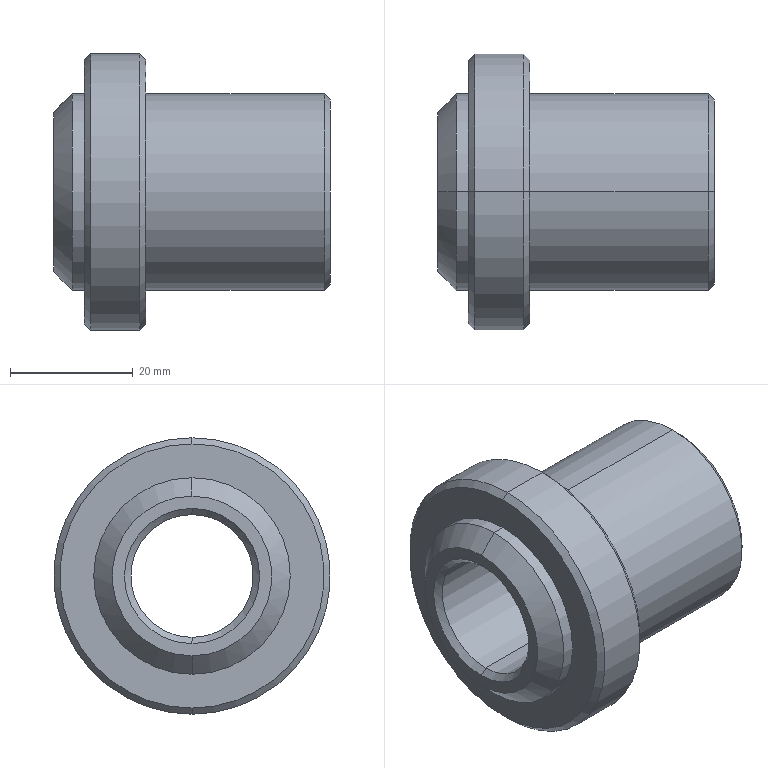Part | SolidWorks | features Chamfer 2, Revolution 1 | 1 solid | 24 faces | box 45 x 45 x 45 mm | volume 29238 mm3 | cone 12 | cylinder 8 | plane 4 | commonest cylinder face diameters 32 x4 20 x2 45 x2
STEP:
#1=CARTESIAN_POINT('',(-45.,0.,13.));
#2=VERTEX_POINT('',#1);
#3=CARTESIAN_POINT('',(-45.,0.,-13.));
#4=VERTEX_POINT('',#3);
#5=CARTESIAN_POINT('',(-45.,0.,0.));
#6=DIRECTION('',(-1.,0.,0.));
#7=DIRECTION('',(0.,0.,1.));
#8=AXIS2_PLACEMENT_3D('',#5,#6,#7);
#9=CIRCLE('',#8,13.);
#10=EDGE_CURVE('',#2,#4,#9,.T.);
#11=ORIENTED_EDGE('',*,*,#10,.F.);
#12=CARTESIAN_POINT('',(-42.,0.,16.));
#13=VERTEX_POINT('',#12);
#14=CARTESIAN_POINT('',(-42.,0.,16.));
#15=DIRECTION('',(0.7071,0.,0.7071));
#16=VECTOR('',#15,1000.);
#17=LINE('',#14,#16);
#18=EDGE_CURVE('',#2,#13,#17,.T.);
#19=ORIENTED_EDGE('',*,*,#18,.T.);
#20=CARTESIAN_POINT('',(-42.,0.,-16.));
#21=VERTEX_POINT('',#20);
#22=CARTESIAN_POINT('',(-42.,0.,0.));
#23=DIRECTION('',(1.,0.,0.));
#24=DIRECTION('',(0.,0.,1.));
#25=AXIS2_PLACEMENT_3D('',#22,#23,#24);
#26=CIRCLE('',#25,16.);
#27=EDGE_CURVE('',#21,#13,#26,.T.);
#28=ORIENTED_EDGE('',*,*,#27,.F.);
#29=CARTESIAN_POINT('',(-42.,0.,-16.));
#30=DIRECTION('',(0.7071,0.,-0.7071));
#31=VECTOR('',#30,1000.);
#32=LINE('',#29,#31);
#33=EDGE_CURVE('',#4,#21,#32,.T.);
#34=ORIENTED_EDGE('',*,*,#33,.F.);
#35=EDGE_LOOP('',(#11,#19,#28,#34));
#36=FACE_OUTER_BOUND('',#35,.T.);
#37=CARTESIAN_POINT('',(-42.,0.,0.));
#38=DIRECTION('',(1.,0.,0.));
#39=DIRECTION('',(0.,0.,-1.));
#40=AXIS2_PLACEMENT_3D('',#37,#38,#39);
#41=CONICAL_SURFACE('',#40,16.,0.7854);
#42=ADVANCED_FACE('',(#36),#41,.T.);
#43=CARTESIAN_POINT('',(-40.,0.,21.5));
#44=VERTEX_POINT('',#43);
#45=CARTESIAN_POINT('',(-40.,0.,-21.5));
#46=VERTEX_POINT('',#45);
#47=CARTESIAN_POINT('',(-40.,0.,0.));
#48=DIRECTION('',(-1.,0.,0.));
#49=DIRECTION('',(0.,0.,1.));
#50=AXIS2_PLACEMENT_3D('',#47,#48,#49);
#51=CIRCLE('',#50,21.5);
#52=EDGE_CURVE('',#44,#46,#51,.T.);
#53=ORIENTED_EDGE('',*,*,#52,.F.);
#54=CARTESIAN_POINT('',(-39.,0.,22.5));
#55=VERTEX_POINT('',#54);
#56=CARTESIAN_POINT('',(-39.,0.,22.5));
#57=DIRECTION('',(0.7071,0.,0.7071));
#58=VECTOR('',#57,1000.);
#59=LINE('',#56,#58);
#60=EDGE_CURVE('',#44,#55,#59,.T.);
#61=ORIENTED_EDGE('',*,*,#60,.T.);
#62=CARTESIAN_POINT('',(-39.,0.,-22.5));
#63=VERTEX_POINT('',#62);
#64=CARTESIAN_POINT('',(-39.,0.,0.));
#65=DIRECTION('',(1.,0.,0.));
#66=DIRECTION('',(0.,0.,1.));
#67=AXIS2_PLACEMENT_3D('',#64,#65,#66);
#68=CIRCLE('',#67,22.5);
#69=EDGE_CURVE('',#63,#55,#68,.T.);
#70=ORIENTED_EDGE('',*,*,#69,.F.);
#71=CARTESIAN_POINT('',(-39.,0.,-22.5));
#72=DIRECTION('',(0.7071,0.,-0.7071));
#73=VECTOR('',#72,1000.);
#74=LINE('',#71,#73);
#75=EDGE_CURVE('',#46,#63,#74,.T.);
#76=ORIENTED_EDGE('',*,*,#75,.F.);
#77=EDGE_LOOP('',(#53,#61,#70,#76));
#78=FACE_OUTER_BOUND('',#77,.T.);
#79=CARTESIAN_POINT('',(-39.,0.,0.));
#80=DIRECTION('',(1.,0.,0.));
#81=DIRECTION('',(0.,0.,-1.));
#82=AXIS2_PLACEMENT_3D('',#79,#80,#81);
#83=CONICAL_SURFACE('',#82,22.5,0.7854);
#84=ADVANCED_FACE('',(#78),#83,.T.);
#85=CARTESIAN_POINT('',(-30.,0.,-21.5));
#86=VERTEX_POINT('',#85);
#87=CARTESIAN_POINT('',(-30.,0.,21.5));
#88=VERTEX_POINT('',#87);
#89=CARTESIAN_POINT('',(-30.,0.,0.));
#90=DIRECTION('',(1.,0.,0.));
#91=DIRECTION('',(0.,0.,-1.));
#92=AXIS2_PLACEMENT_3D('',#89,#90,#91);
#93=CIRCLE('',#92,21.5);
#94=EDGE_CURVE('',#86,#88,#93,.T.);
#95=ORIENTED_EDGE('',*,*,#94,.F.);
#96=CARTESIAN_POINT('',(-31.,0.,-22.5));
#97=VERTEX_POINT('',#96);
#98=CARTESIAN_POINT('',(-30.,0.,-21.5));
#99=DIRECTION('',(-0.7071,0.,-0.7071));
#100=VECTOR('',#99,1000.);
#101=LINE('',#98,#100);
#102=EDGE_CURVE('',#86,#97,#101,.T.);
#103=ORIENTED_EDGE('',*,*,#102,.T.);
#104=CARTESIAN_POINT('',(-31.,0.,22.5));
#105=VERTEX_POINT('',#104);
#106=CARTESIAN_POINT('',(-31.,0.,0.));
#107=DIRECTION('',(-1.,0.,0.));
#108=DIRECTION('',(0.,0.,-1.));
#109=AXIS2_PLACEMENT_3D('',#106,#107,#108);
#110=CIRCLE('',#109,22.5);
#111=EDGE_CURVE('',#105,#97,#110,.T.);
#112=ORIENTED_EDGE('',*,*,#111,.F.);
#113=CARTESIAN_POINT('',(-30.,0.,21.5));
#114=DIRECTION('',(-0.7071,0.,0.7071));
#115=VECTOR('',#114,1000.);
#116=LINE('',#113,#115);
#117=EDGE_CURVE('',#88,#105,#116,.T.);
#118=ORIENTED_EDGE('',*,*,#117,.F.);
#119=EDGE_LOOP('',(#95,#103,#112,#118));
#120=FACE_OUTER_BOUND('',#119,.T.);
#121=CARTESIAN_POINT('',(-30.,0.,0.));
#122=DIRECTION('',(-1.,0.,0.));
#123=DIRECTION('',(0.,0.,1.));
#124=AXIS2_PLACEMENT_3D('',#121,#122,#123);
#125=CONICAL_SURFACE('',#124,21.5,0.7854);
#126=ADVANCED_FACE('',(#120),#125,.T.);
#127=CARTESIAN_POINT('',(0.,0.,-15.));
#128=VERTEX_POINT('',#127);
#129=CARTESIAN_POINT('',(0.,0.,15.));
#130=VERTEX_POINT('',#129);
#131=CARTESIAN_POINT('',(0.,0.,0.));
#132=DIRECTION('',(1.,0.,0.));
#133=DIRECTION('',(0.,0.,-1.));
#134=AXIS2_PLACEMENT_3D('',#131,#132,#133);
#135=CIRCLE('',#134,15.);
#136=EDGE_CURVE('',#128,#130,#135,.T.);
#137=ORIENTED_EDGE('',*,*,#136,.F.);
#138=CARTESIAN_POINT('',(-1.,0.,-16.));
#139=VERTEX_POINT('',#138);
#140=CARTESIAN_POINT('',(0.,0.,-15.));
#141=DIRECTION('',(-0.7071,0.,-0.7071));
#142=VECTOR('',#141,1000.);
#143=LINE('',#140,#142);
#144=EDGE_CURVE('',#128,#139,#143,.T.);
#145=ORIENTED_EDGE('',*,*,#144,.T.);
#146=CARTESIAN_POINT('',(-1.,0.,16.));
#147=VERTEX_POINT('',#146);
#148=CARTESIAN_POINT('',(-1.,0.,0.));
#149=DIRECTION('',(-1.,0.,0.));
#150=DIRECTION('',(0.,0.,-1.));
#151=AXIS2_PLACEMENT_3D('',#148,#149,#150);
#152=CIRCLE('',#151,16.);
#153=EDGE_CURVE('',#147,#139,#152,.T.);
#154=ORIENTED_EDGE('',*,*,#153,.F.);
#155=CARTESIAN_POINT('',(0.,0.,15.));
#156=DIRECTION('',(-0.7071,0.,0.7071));
#157=VECTOR('',#156,1000.);
#158=LINE('',#155,#157);
#159=EDGE_CURVE('',#130,#147,#158,.T.);
#160=ORIENTED_EDGE('',*,*,#159,.F.);
#161=EDGE_LOOP('',(#137,#145,#154,#160));
#162=FACE_OUTER_BOUND('',#161,.T.);
#163=CARTESIAN_POINT('',(0.,0.,0.));
#164=DIRECTION('',(-1.,0.,0.));
#165=DIRECTION('',(0.,0.,1.));
#166=AXIS2_PLACEMENT_3D('',#163,#164,#165);
#167=CONICAL_SURFACE('',#166,15.,0.7854);
#168=ADVANCED_FACE('',(#162),#167,.T.);
#169=CARTESIAN_POINT('',(-1.,0.,10.));
#170=VERTEX_POINT('',#169);
#171=CARTESIAN_POINT('',(-1.,0.,-10.));
#172=VERTEX_POINT('',#171);
#173=CARTESIAN_POINT('',(-1.,0.,0.));
#174=DIRECTION('',(1.,0.,0.));
#175=DIRECTION('',(0.,0.,-1.));
#176=AXIS2_PLACEMENT_3D('',#173,#174,#175);
#177=CIRCLE('',#176,10.);
#178=EDGE_CURVE('',#170,#172,#177,.T.);
#179=ORIENTED_EDGE('',*,*,#178,.F.);
#180=CARTESIAN_POINT('',(0.,0.,11.));
#181=VERTEX_POINT('',#180);
#182=CARTESIAN_POINT('',(-1.,0.,10.));
#183=DIRECTION('',(0.7071,0.,0.7071));
#184=VECTOR('',#183,1000.);
#185=LINE('',#182,#184);
#186=EDGE_CURVE('',#170,#181,#185,.T.);
#187=ORIENTED_EDGE('',*,*,#186,.T.);
#188=CARTESIAN_POINT('',(0.,0.,-11.));
#189=VERTEX_POINT('',#188);
#190=CARTESIAN_POINT('',(0.,0.,0.));
#191=DIRECTION('',(-1.,0.,0.));
#192=DIRECTION('',(0.,0.,-1.));
#193=AXIS2_PLACEMENT_3D('',#190,#191,#192);
#194=CIRCLE('',#193,11.);
#195=EDGE_CURVE('',#189,#181,#194,.T.);
#196=ORIENTED_EDGE('',*,*,#195,.F.);
#197=CARTESIAN_POINT('',(-1.,0.,-10.));
#198=DIRECTION('',(0.7071,0.,-0.7071));
#199=VECTOR('',#198,1000.);
#200=LINE('',#197,#199);
#201=EDGE_CURVE('',#172,#189,#200,.T.);
#202=ORIENTED_EDGE('',*,*,#201,.F.);
#203=EDGE_LOOP('',(#179,#187,#196,#202));
#204=FACE_OUTER_BOUND('',#203,.T.);
#205=CARTESIAN_POINT('',(-1.,0.,0.));
#206=DIRECTION('',(1.,0.,0.));
#207=DIRECTION('',(0.,0.,-1.));
#208=AXIS2_PLACEMENT_3D('',#205,#206,#207);
#209=CONICAL_SURFACE('',#208,10.,0.7854);
#210=ADVANCED_FACE('',(#204),#209,.F.);
#211=CARTESIAN_POINT('',(-44.,0.,-10.));
#212=VERTEX_POINT('',#211);
#213=CARTESIAN_POINT('',(-44.,0.,10.));
#214=VERTEX_POINT('',#213);
#215=CARTESIAN_POINT('',(-44.,0.,0.));
#216=DIRECTION('',(-1.,0.,0.));
#217=DIRECTION('',(0.,0.,1.));
#218=AXIS2_PLACEMENT_3D('',#215,#216,#217);
#219=CIRCLE('',#218,10.);
#220=EDGE_CURVE('',#212,#214,#219,.T.);
#221=ORIENTED_EDGE('',*,*,#220,.F.);
#222=CARTESIAN_POINT('',(-45.,0.,-11.));
#223=VERTEX_POINT('',#222);
#224=CARTESIAN_POINT('',(-45.,0.,-11.));
#225=DIRECTION('',(-0.7071,0.,-0.7071));
#226=VECTOR('',#225,1000.);
#227=LINE('',#224,#226);
#228=EDGE_CURVE('',#212,#223,#227,.T.);
#229=ORIENTED_EDGE('',*,*,#228,.T.);
#230=CARTESIAN_POINT('',(-45.,0.,11.));
#231=VERTEX_POINT('',#230);
#232=CARTESIAN_POINT('',(-45.,0.,0.));
#233=DIRECTION('',(1.,0.,0.));
#234=DIRECTION('',(0.,0.,1.));
#235=AXIS2_PLACEMENT_3D('',#232,#233,#234);
#236=CIRCLE('',#235,11.);
#237=EDGE_CURVE('',#231,#223,#236,.T.);
#238=ORIENTED_EDGE('',*,*,#237,.F.);
#239=CARTESIAN_POINT('',(-45.,0.,11.));
#240=DIRECTION('',(-0.7071,0.,0.7071));
#241=VECTOR('',#240,1000.);
#242=LINE('',#239,#241);
#243=EDGE_CURVE('',#214,#231,#242,.T.);
#244=ORIENTED_EDGE('',*,*,#243,.F.);
#245=EDGE_LOOP('',(#221,#229,#238,#244));
#246=FACE_OUTER_BOUND('',#245,.T.);
#247=CARTESIAN_POINT('',(-45.,0.,0.));
#248=DIRECTION('',(-1.,0.,0.));
#249=DIRECTION('',(0.,0.,1.));
#250=AXIS2_PLACEMENT_3D('',#247,#248,#249);
#251=CONICAL_SURFACE('',#250,11.,0.7854);
#252=ADVANCED_FACE('',(#246),#251,.F.);
#253=ORIENTED_EDGE('',*,*,#69,.T.);
#254=CARTESIAN_POINT('',(0.,0.,22.5));
#255=DIRECTION('',(1.,0.,0.));
#256=VECTOR('',#255,1000.);
#257=LINE('',#254,#256);
#258=EDGE_CURVE('',#55,#105,#257,.T.);
#259=ORIENTED_EDGE('',*,*,#258,.T.);
#260=ORIENTED_EDGE('',*,*,#111,.T.);
#261=CARTESIAN_POINT('',(0.,0.,-22.5));
#262=DIRECTION('',(1.,0.,0.));
#263=VECTOR('',#262,1000.);
#264=LINE('',#261,#263);
#265=EDGE_CURVE('',#63,#97,#264,.T.);
#266=ORIENTED_EDGE('',*,*,#265,.F.);
#267=EDGE_LOOP('',(#253,#259,#260,#266));
#268=FACE_OUTER_BOUND('',#267,.T.);
#269=CARTESIAN_POINT('',(0.,0.,0.));
#270=DIRECTION('',(1.,0.,0.));
#271=DIRECTION('',(0.,0.,-1.));
#272=AXIS2_PLACEMENT_3D('',#269,#270,#271);
#273=CYLINDRICAL_SURFACE('',#272,22.5);
#274=ADVANCED_FACE('',(#268),#273,.T.);
#275=ORIENTED_EDGE('',*,*,#27,.T.);
#276=CARTESIAN_POINT('',(-40.,0.,16.));
#277=VERTEX_POINT('',#276);
#278=CARTESIAN_POINT('',(0.,0.,16.));
#279=DIRECTION('',(1.,0.,0.));
#280=VECTOR('',#279,1000.);
#281=LINE('',#278,#280);
#282=EDGE_CURVE('',#13,#277,#281,.T.);
#283=ORIENTED_EDGE('',*,*,#282,.T.);
#284=CARTESIAN_POINT('',(-40.,0.,-16.));
#285=VERTEX_POINT('',#284);
#286=CARTESIAN_POINT('',(-40.,0.,0.));
#287=DIRECTION('',(1.,0.,0.));
#288=DIRECTION('',(0.,0.,-1.));
#289=AXIS2_PLACEMENT_3D('',#286,#287,#288);
#290=CIRCLE('',#289,16.);
#291=EDGE_CURVE('',#285,#277,#290,.T.);
#292=ORIENTED_EDGE('',*,*,#291,.F.);
#293=CARTESIAN_POINT('',(0.,0.,-16.));
#294=DIRECTION('',(1.,0.,0.));
#295=VECTOR('',#294,1000.);
#296=LINE('',#293,#295);
#297=EDGE_CURVE('',#21,#285,#296,.T.);
#298=ORIENTED_EDGE('',*,*,#297,.F.);
#299=EDGE_LOOP('',(#275,#283,#292,#298));
#300=FACE_OUTER_BOUND('',#299,.T.);
#301=CARTESIAN_POINT('',(0.,0.,0.));
#302=DIRECTION('',(1.,0.,0.));
#303=DIRECTION('',(0.,0.,-1.));
#304=AXIS2_PLACEMENT_3D('',#301,#302,#303);
#305=CYLINDRICAL_SURFACE('',#304,16.);
#306=ADVANCED_FACE('',(#300),#305,.T.);
#307=ORIENTED_EDGE('',*,*,#220,.T.);
#308=CARTESIAN_POINT('',(0.,0.,10.));
#309=DIRECTION('',(1.,0.,0.));
#310=VECTOR('',#309,1000.);
#311=LINE('',#308,#310);
#312=EDGE_CURVE('',#214,#170,#311,.T.);
#313=ORIENTED_EDGE('',*,*,#312,.T.);
#314=ORIENTED_EDGE('',*,*,#178,.T.);
#315=CARTESIAN_POINT('',(0.,0.,-10.));
#316=DIRECTION('',(1.,0.,0.));
#317=VECTOR('',#316,1000.);
#318=LINE('',#315,#317);
#319=EDGE_CURVE('',#212,#172,#318,.T.);
#320=ORIENTED_EDGE('',*,*,#319,.F.);
#321=EDGE_LOOP('',(#307,#313,#314,#320));
#322=FACE_OUTER_BOUND('',#321,.T.);
#323=CARTESIAN_POINT('',(0.,0.,0.));
#324=DIRECTION('',(1.,0.,0.));
#325=DIRECTION('',(0.,0.,-1.));
#326=AXIS2_PLACEMENT_3D('',#323,#324,#325);
#327=CYLINDRICAL_SURFACE('',#326,10.);
#328=ADVANCED_FACE('',(#322),#327,.F.);
#329=CARTESIAN_POINT('',(-30.,0.,-16.));
#330=VERTEX_POINT('',#329);
#331=CARTESIAN_POINT('',(-30.,0.,16.));
#332=VERTEX_POINT('',#331);
#333=CARTESIAN_POINT('',(-30.,0.,0.));
#334=DIRECTION('',(1.,0.,0.));
#335=DIRECTION('',(0.,0.,-1.));
#336=AXIS2_PLACEMENT_3D('',#333,#334,#335);
#337=CIRCLE('',#336,16.);
#338=EDGE_CURVE('',#330,#332,#337,.T.);
#339=ORIENTED_EDGE('',*,*,#338,.T.);
#340=CARTESIAN_POINT('',(0.,0.,16.));
#341=DIRECTION('',(1.,0.,0.));
#342=VECTOR('',#341,1000.);
#343=LINE('',#340,#342);
#344=EDGE_CURVE('',#332,#147,#343,.T.);
#345=ORIENTED_EDGE('',*,*,#344,.T.);
#346=ORIENTED_EDGE('',*,*,#153,.T.);
#347=CARTESIAN_POINT('',(0.,0.,-16.));
#348=DIRECTION('',(1.,0.,0.));
#349=VECTOR('',#348,1000.);
#350=LINE('',#347,#349);
#351=EDGE_CURVE('',#330,#139,#350,.T.);
#352=ORIENTED_EDGE('',*,*,#351,.F.);
#353=EDGE_LOOP('',(#339,#345,#346,#352));
#354=FACE_OUTER_BOUND('',#353,.T.);
#355=CARTESIAN_POINT('',(0.,0.,0.));
#356=DIRECTION('',(1.,0.,0.));
#357=DIRECTION('',(0.,0.,-1.));
#358=AXIS2_PLACEMENT_3D('',#355,#356,#357);
#359=CYLINDRICAL_SURFACE('',#358,16.);
#360=ADVANCED_FACE('',(#354),#359,.T.);
#361=ORIENTED_EDGE('',*,*,#344,.F.);
#362=CARTESIAN_POINT('',(-30.,0.,0.));
#363=DIRECTION('',(1.,0.,0.));
#364=DIRECTION('',(0.,0.,-1.));
#365=AXIS2_PLACEMENT_3D('',#362,#363,#364);
#366=CIRCLE('',#365,16.);
#367=EDGE_CURVE('',#332,#330,#366,.T.);
#368=ORIENTED_EDGE('',*,*,#367,.T.);
#369=ORIENTED_EDGE('',*,*,#351,.T.);
#370=CARTESIAN_POINT('',(-1.,0.,0.));
#371=DIRECTION('',(-1.,0.,0.));
#372=DIRECTION('',(0.,0.,-1.));
#373=AXIS2_PLACEMENT_3D('',#370,#371,#372);
#374=CIRCLE('',#373,16.);
#375=EDGE_CURVE('',#139,#147,#374,.T.);
#376=ORIENTED_EDGE('',*,*,#375,.T.);
#377=EDGE_LOOP('',(#361,#368,#369,#376));
#378=FACE_OUTER_BOUND('',#377,.T.);
#379=CARTESIAN_POINT('',(0.,0.,0.));
#380=DIRECTION('',(1.,0.,0.));
#381=DIRECTION('',(0.,0.,-1.));
#382=AXIS2_PLACEMENT_3D('',#379,#380,#381);
#383=CYLINDRICAL_SURFACE('',#382,16.);
#384=ADVANCED_FACE('',(#378),#383,.T.);
#385=ORIENTED_EDGE('',*,*,#195,.T.);
#386=CARTESIAN_POINT('',(0.,0.,0.));
#387=DIRECTION('',(-1.,0.,0.));
#388=DIRECTION('',(0.,0.,-1.));
#389=AXIS2_PLACEMENT_3D('',#386,#387,#388);
#390=CIRCLE('',#389,11.);
#391=EDGE_CURVE('',#181,#189,#390,.T.);
#392=ORIENTED_EDGE('',*,*,#391,.T.);
#393=EDGE_LOOP('',(#385,#392));
#394=FACE_BOUND('',#393,.T.);
#395=CARTESIAN_POINT('',(0.,0.,0.));
#396=DIRECTION('',(1.,0.,0.));
#397=DIRECTION('',(0.,0.,-1.));
#398=AXIS2_PLACEMENT_3D('',#395,#396,#397);
#399=CIRCLE('',#398,15.);
#400=EDGE_CURVE('',#130,#128,#399,.T.);
#401=ORIENTED_EDGE('',*,*,#400,.T.);
#402=ORIENTED_EDGE('',*,*,#136,.T.);
#403=EDGE_LOOP('',(#401,#402));
#404=FACE_OUTER_BOUND('',#403,.T.);
#405=CARTESIAN_POINT('',(0.,10.,0.));
#406=DIRECTION('',(1.,0.,0.));
#407=DIRECTION('',(0.,0.,-1.));
#408=AXIS2_PLACEMENT_3D('',#405,#406,#407);
#409=PLANE('',#408);
#410=ADVANCED_FACE('',(#394,#404),#409,.T.);
#411=ORIENTED_EDGE('',*,*,#312,.F.);
#412=CARTESIAN_POINT('',(-44.,0.,0.));
#413=DIRECTION('',(-1.,0.,0.));
#414=DIRECTION('',(0.,0.,1.));
#415=AXIS2_PLACEMENT_3D('',#412,#413,#414);
#416=CIRCLE('',#415,10.);
#417=EDGE_CURVE('',#214,#212,#416,.T.);
#418=ORIENTED_EDGE('',*,*,#417,.T.);
#419=ORIENTED_EDGE('',*,*,#319,.T.);
#420=CARTESIAN_POINT('',(-1.,0.,0.));
#421=DIRECTION('',(1.,0.,0.));
#422=DIRECTION('',(0.,0.,-1.));
#423=AXIS2_PLACEMENT_3D('',#420,#421,#422);
#424=CIRCLE('',#423,10.);
#425=EDGE_CURVE('',#172,#170,#424,.T.);
#426=ORIENTED_EDGE('',*,*,#425,.T.);
#427=EDGE_LOOP('',(#411,#418,#419,#426));
#428=FACE_OUTER_BOUND('',#427,.T.);
#429=CARTESIAN_POINT('',(0.,0.,0.));
#430=DIRECTION('',(1.,0.,0.));
#431=DIRECTION('',(0.,0.,-1.));
#432=AXIS2_PLACEMENT_3D('',#429,#430,#431);
#433=CYLINDRICAL_SURFACE('',#432,10.);
#434=ADVANCED_FACE('',(#428),#433,.F.);
#435=CARTESIAN_POINT('',(-45.,0.,0.));
#436=DIRECTION('',(-1.,0.,0.));
#437=DIRECTION('',(0.,0.,1.));
#438=AXIS2_PLACEMENT_3D('',#435,#436,#437);
#439=CIRCLE('',#438,13.);
#440=EDGE_CURVE('',#4,#2,#439,.T.);
#441=ORIENTED_EDGE('',*,*,#440,.T.);
#442=ORIENTED_EDGE('',*,*,#10,.T.);
#443=EDGE_LOOP('',(#441,#442));
#444=FACE_OUTER_BOUND('',#443,.T.);
#445=ORIENTED_EDGE('',*,*,#237,.T.);
#446=CARTESIAN_POINT('',(-45.,0.,0.));
#447=DIRECTION('',(1.,0.,0.));
#448=DIRECTION('',(0.,0.,1.));
#449=AXIS2_PLACEMENT_3D('',#446,#447,#448);
#450=CIRCLE('',#449,11.);
#451=EDGE_CURVE('',#223,#231,#450,.T.);
#452=ORIENTED_EDGE('',*,*,#451,.T.);
#453=EDGE_LOOP('',(#445,#452));
#454=FACE_BOUND('',#453,.T.);
#455=CARTESIAN_POINT('',(-45.,16.,0.));
#456=DIRECTION('',(-1.,0.,0.));
#457=DIRECTION('',(0.,0.,1.));
#458=AXIS2_PLACEMENT_3D('',#455,#456,#457);
#459=PLANE('',#458);
#460=ADVANCED_FACE('',(#444,#454),#459,.T.);
#461=ORIENTED_EDGE('',*,*,#282,.F.);
#462=CARTESIAN_POINT('',(-42.,0.,0.));
#463=DIRECTION('',(1.,0.,0.));
#464=DIRECTION('',(0.,0.,1.));
#465=AXIS2_PLACEMENT_3D('',#462,#463,#464);
#466=CIRCLE('',#465,16.);
#467=EDGE_CURVE('',#13,#21,#466,.T.);
#468=ORIENTED_EDGE('',*,*,#467,.T.);
#469=ORIENTED_EDGE('',*,*,#297,.T.);
#470=CARTESIAN_POINT('',(-40.,0.,0.));
#471=DIRECTION('',(1.,0.,0.));
#472=DIRECTION('',(0.,0.,-1.));
#473=AXIS2_PLACEMENT_3D('',#470,#471,#472);
#474=CIRCLE('',#473,16.);
#475=EDGE_CURVE('',#277,#285,#474,.T.);
#476=ORIENTED_EDGE('',*,*,#475,.F.);
#477=EDGE_LOOP('',(#461,#468,#469,#476));
#478=FACE_OUTER_BOUND('',#477,.T.);
#479=CARTESIAN_POINT('',(0.,0.,0.));
#480=DIRECTION('',(1.,0.,0.));
#481=DIRECTION('',(0.,0.,-1.));
#482=AXIS2_PLACEMENT_3D('',#479,#480,#481);
#483=CYLINDRICAL_SURFACE('',#482,16.);
#484=ADVANCED_FACE('',(#478),#483,.T.);
#485=CARTESIAN_POINT('',(-40.,0.,0.));
#486=DIRECTION('',(-1.,0.,0.));
#487=DIRECTION('',(0.,0.,1.));
#488=AXIS2_PLACEMENT_3D('',#485,#486,#487);
#489=CIRCLE('',#488,21.5);
#490=EDGE_CURVE('',#46,#44,#489,.T.);
#491=ORIENTED_EDGE('',*,*,#490,.T.);
#492=ORIENTED_EDGE('',*,*,#52,.T.);
#493=EDGE_LOOP('',(#491,#492));
#494=FACE_OUTER_BOUND('',#493,.T.);
#495=ORIENTED_EDGE('',*,*,#291,.T.);
#496=ORIENTED_EDGE('',*,*,#475,.T.);
#497=EDGE_LOOP('',(#495,#496));
#498=FACE_BOUND('',#497,.T.);
#499=CARTESIAN_POINT('',(-40.,22.5,0.));
#500=DIRECTION('',(-1.,0.,0.));
#501=DIRECTION('',(0.,0.,1.));
#502=AXIS2_PLACEMENT_3D('',#499,#500,#501);
#503=PLANE('',#502);
#504=ADVANCED_FACE('',(#494,#498),#503,.T.);
#505=ORIENTED_EDGE('',*,*,#258,.F.);
#506=CARTESIAN_POINT('',(-39.,0.,0.));
#507=DIRECTION('',(1.,0.,0.));
#508=DIRECTION('',(0.,0.,1.));
#509=AXIS2_PLACEMENT_3D('',#506,#507,#508);
#510=CIRCLE('',#509,22.5);
#511=EDGE_CURVE('',#55,#63,#510,.T.);
#512=ORIENTED_EDGE('',*,*,#511,.T.);
#513=ORIENTED_EDGE('',*,*,#265,.T.);
#514=CARTESIAN_POINT('',(-31.,0.,0.));
#515=DIRECTION('',(-1.,0.,0.));
#516=DIRECTION('',(0.,0.,-1.));
#517=AXIS2_PLACEMENT_3D('',#514,#515,#516);
#518=CIRCLE('',#517,22.5);
#519=EDGE_CURVE('',#97,#105,#518,.T.);
#520=ORIENTED_EDGE('',*,*,#519,.T.);
#521=EDGE_LOOP('',(#505,#512,#513,#520));
#522=FACE_OUTER_BOUND('',#521,.T.);
#523=CARTESIAN_POINT('',(0.,0.,0.));
#524=DIRECTION('',(1.,0.,0.));
#525=DIRECTION('',(0.,0.,-1.));
#526=AXIS2_PLACEMENT_3D('',#523,#524,#525);
#527=CYLINDRICAL_SURFACE('',#526,22.5);
#528=ADVANCED_FACE('',(#522),#527,.T.);
#529=CARTESIAN_POINT('',(-30.,0.,0.));
#530=DIRECTION('',(1.,0.,0.));
#531=DIRECTION('',(0.,0.,-1.));
#532=AXIS2_PLACEMENT_3D('',#529,#530,#531);
#533=CIRCLE('',#532,21.5);
#534=EDGE_CURVE('',#88,#86,#533,.T.);
#535=ORIENTED_EDGE('',*,*,#534,.T.);
#536=ORIENTED_EDGE('',*,*,#94,.T.);
#537=EDGE_LOOP('',(#535,#536));
#538=FACE_OUTER_BOUND('',#537,.T.);
#539=ORIENTED_EDGE('',*,*,#338,.F.);
#540=ORIENTED_EDGE('',*,*,#367,.F.);
#541=EDGE_LOOP('',(#539,#540));
#542=FACE_BOUND('',#541,.T.);
#543=CARTESIAN_POINT('',(-30.,16.,0.));
#544=DIRECTION('',(1.,0.,0.));
#545=DIRECTION('',(0.,0.,-1.));
#546=AXIS2_PLACEMENT_3D('',#543,#544,#545);
#547=PLANE('',#546);
#548=ADVANCED_FACE('',(#538,#542),#547,.T.);
#549=ORIENTED_EDGE('',*,*,#228,.F.);
#550=ORIENTED_EDGE('',*,*,#417,.F.);
#551=ORIENTED_EDGE('',*,*,#243,.T.);
#552=ORIENTED_EDGE('',*,*,#451,.F.);
#553=EDGE_LOOP('',(#549,#550,#551,#552));
#554=FACE_OUTER_BOUND('',#553,.T.);
#555=CARTESIAN_POINT('',(-45.,0.,0.));
#556=DIRECTION('',(-1.,0.,0.));
#557=DIRECTION('',(0.,0.,1.));
#558=AXIS2_PLACEMENT_3D('',#555,#556,#557);
#559=CONICAL_SURFACE('',#558,11.,0.7854);
#560=ADVANCED_FACE('',(#554),#559,.F.);
#561=ORIENTED_EDGE('',*,*,#186,.F.);
#562=ORIENTED_EDGE('',*,*,#425,.F.);
#563=ORIENTED_EDGE('',*,*,#201,.T.);
#564=ORIENTED_EDGE('',*,*,#391,.F.);
#565=EDGE_LOOP('',(#561,#562,#563,#564));
#566=FACE_OUTER_BOUND('',#565,.T.);
#567=CARTESIAN_POINT('',(-1.,0.,0.));
#568=DIRECTION('',(1.,0.,0.));
#569=DIRECTION('',(0.,0.,-1.));
#570=AXIS2_PLACEMENT_3D('',#567,#568,#569);
#571=CONICAL_SURFACE('',#570,10.,0.7854);
#572=ADVANCED_FACE('',(#566),#571,.F.);
#573=ORIENTED_EDGE('',*,*,#144,.F.);
#574=ORIENTED_EDGE('',*,*,#400,.F.);
#575=ORIENTED_EDGE('',*,*,#159,.T.);
#576=ORIENTED_EDGE('',*,*,#375,.F.);
#577=EDGE_LOOP('',(#573,#574,#575,#576));
#578=FACE_OUTER_BOUND('',#577,.T.);
#579=CARTESIAN_POINT('',(0.,0.,0.));
#580=DIRECTION('',(-1.,0.,0.));
#581=DIRECTION('',(0.,0.,1.));
#582=AXIS2_PLACEMENT_3D('',#579,#580,#581);
#583=CONICAL_SURFACE('',#582,15.,0.7854);
#584=ADVANCED_FACE('',(#578),#583,.T.);
#585=ORIENTED_EDGE('',*,*,#102,.F.);
#586=ORIENTED_EDGE('',*,*,#534,.F.);
#587=ORIENTED_EDGE('',*,*,#117,.T.);
#588=ORIENTED_EDGE('',*,*,#519,.F.);
#589=EDGE_LOOP('',(#585,#586,#587,#588));
#590=FACE_OUTER_BOUND('',#589,.T.);
#591=CARTESIAN_POINT('',(-30.,0.,0.));
#592=DIRECTION('',(-1.,0.,0.));
#593=DIRECTION('',(0.,0.,1.));
#594=AXIS2_PLACEMENT_3D('',#591,#592,#593);
#595=CONICAL_SURFACE('',#594,21.5,0.7854);
#596=ADVANCED_FACE('',(#590),#595,.T.);
#597=ORIENTED_EDGE('',*,*,#60,.F.);
#598=ORIENTED_EDGE('',*,*,#490,.F.);
#599=ORIENTED_EDGE('',*,*,#75,.T.);
#600=ORIENTED_EDGE('',*,*,#511,.F.);
#601=EDGE_LOOP('',(#597,#598,#599,#600));
#602=FACE_OUTER_BOUND('',#601,.T.);
#603=CARTESIAN_POINT('',(-39.,0.,0.));
#604=DIRECTION('',(1.,0.,0.));
#605=DIRECTION('',(0.,0.,-1.));
#606=AXIS2_PLACEMENT_3D('',#603,#604,#605);
#607=CONICAL_SURFACE('',#606,22.5,0.7854);
#608=ADVANCED_FACE('',(#602),#607,.T.);
#609=ORIENTED_EDGE('',*,*,#18,.F.);
#610=ORIENTED_EDGE('',*,*,#440,.F.);
#611=ORIENTED_EDGE('',*,*,#33,.T.);
#612=ORIENTED_EDGE('',*,*,#467,.F.);
#613=EDGE_LOOP('',(#609,#610,#611,#612));
#614=FACE_OUTER_BOUND('',#613,.T.);
#615=CARTESIAN_POINT('',(-42.,0.,0.));
#616=DIRECTION('',(1.,0.,0.));
#617=DIRECTION('',(0.,0.,-1.));
#618=AXIS2_PLACEMENT_3D('',#615,#616,#617);
#619=CONICAL_SURFACE('',#618,16.,0.7854);
#620=ADVANCED_FACE('',(#614),#619,.T.);
#621=CLOSED_SHELL('',(#42,#84,#126,#168,#210,#252,#274,#306,#328,#360,#384,#410,#434,#460,#484,#504,#528,#548,#560,#572,#584,#596,#608,#620));
#622=MANIFOLD_SOLID_BREP('',#621);
#623=CARTESIAN_POINT('',(0.,0.,0.));
#624=DIRECTION('',(0.,0.,1.));
#625=DIRECTION('',(1.,0.,0.));
#626=AXIS2_PLACEMENT_3D('',#623,#624,#625);
#627=(LENGTH_UNIT()NAMED_UNIT(*)SI_UNIT(.MILLI.,.METRE.));
#628=UNCERTAINTY_MEASURE_WITH_UNIT(LENGTH_MEASURE(0.00001),#627,'','');
#629=(NAMED_UNIT(*)PLANE_ANGLE_UNIT()SI_UNIT($,.RADIAN.));
#630=(NAMED_UNIT(*)SI_UNIT($,.STERADIAN.)SOLID_ANGLE_UNIT());
#631=(GEOMETRIC_REPRESENTATION_CONTEXT(3)GLOBAL_UNCERTAINTY_ASSIGNED_CONTEXT((#628))GLOBAL_UNIT_ASSIGNED_CONTEXT((#627,#629,#630))REPRESENTATION_CONTEXT('',''));
#632=ADVANCED_BREP_SHAPE_REPRESENTATION('',(#622,#626),#631);